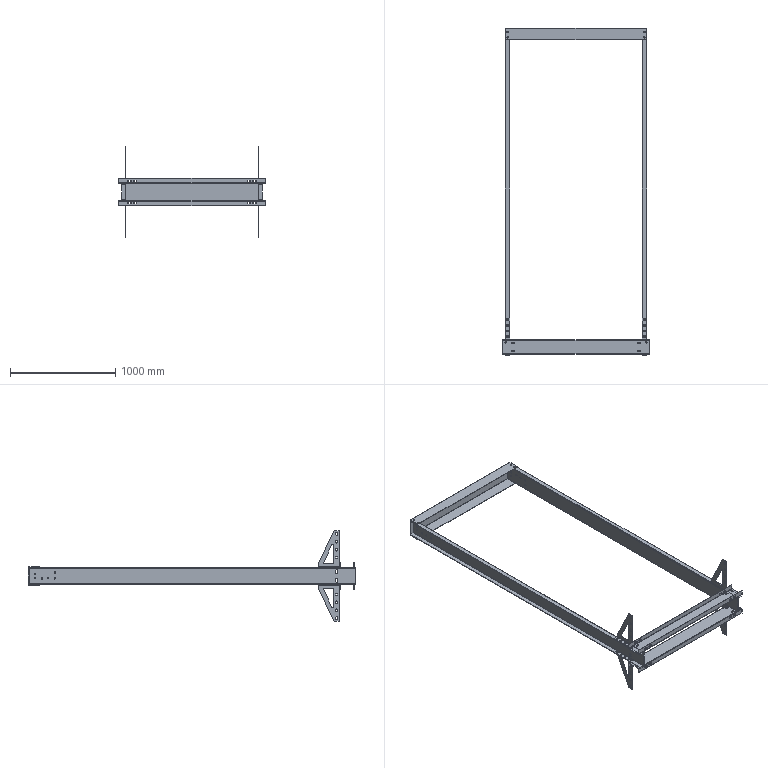Part | 9 solids | 598 faces | box 1390 x 3110 x 860 mm | volume 13259489 mm3 | plane 306 | cylinder 292 | commonest cylinder face diameters 13 x128 14 x108 12 x20 20 x20 2 x12 0.4 x2